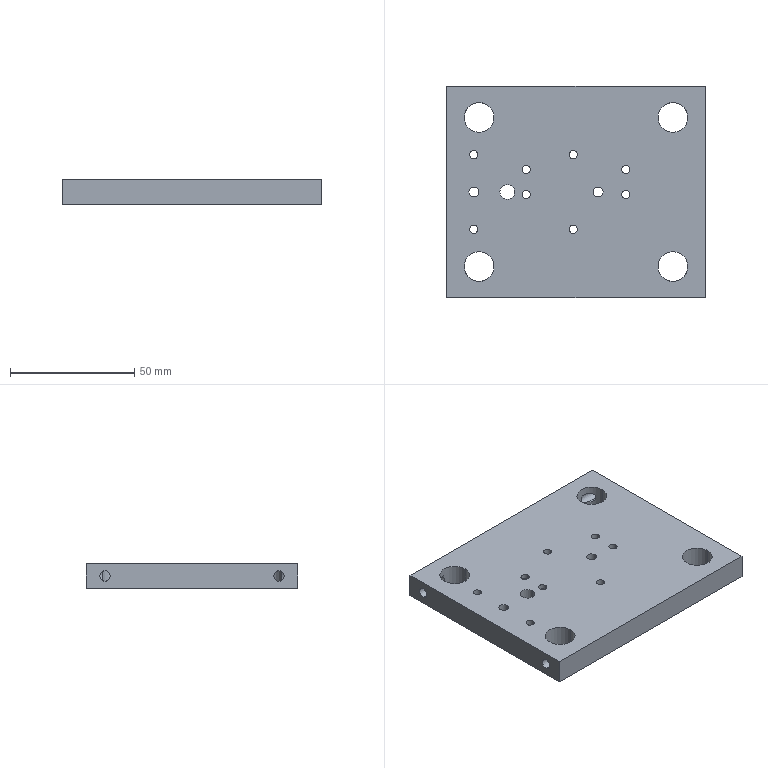Part | STEP file | X77b-01012 | 1 solid | 60 faces | box 103.905 x 85.005 x 10 mm | volume 81895 mm3 | cylinder 46 | plane 10 | cone 4 | commonest cylinder face diameters 3.3 x16 4 x12 4.2 x8 12 x8 6 x2